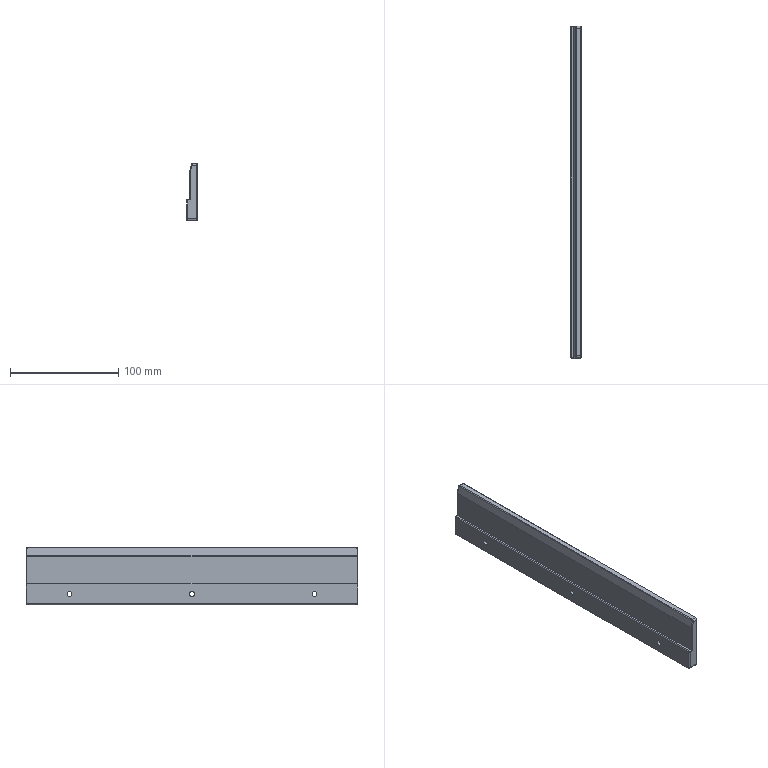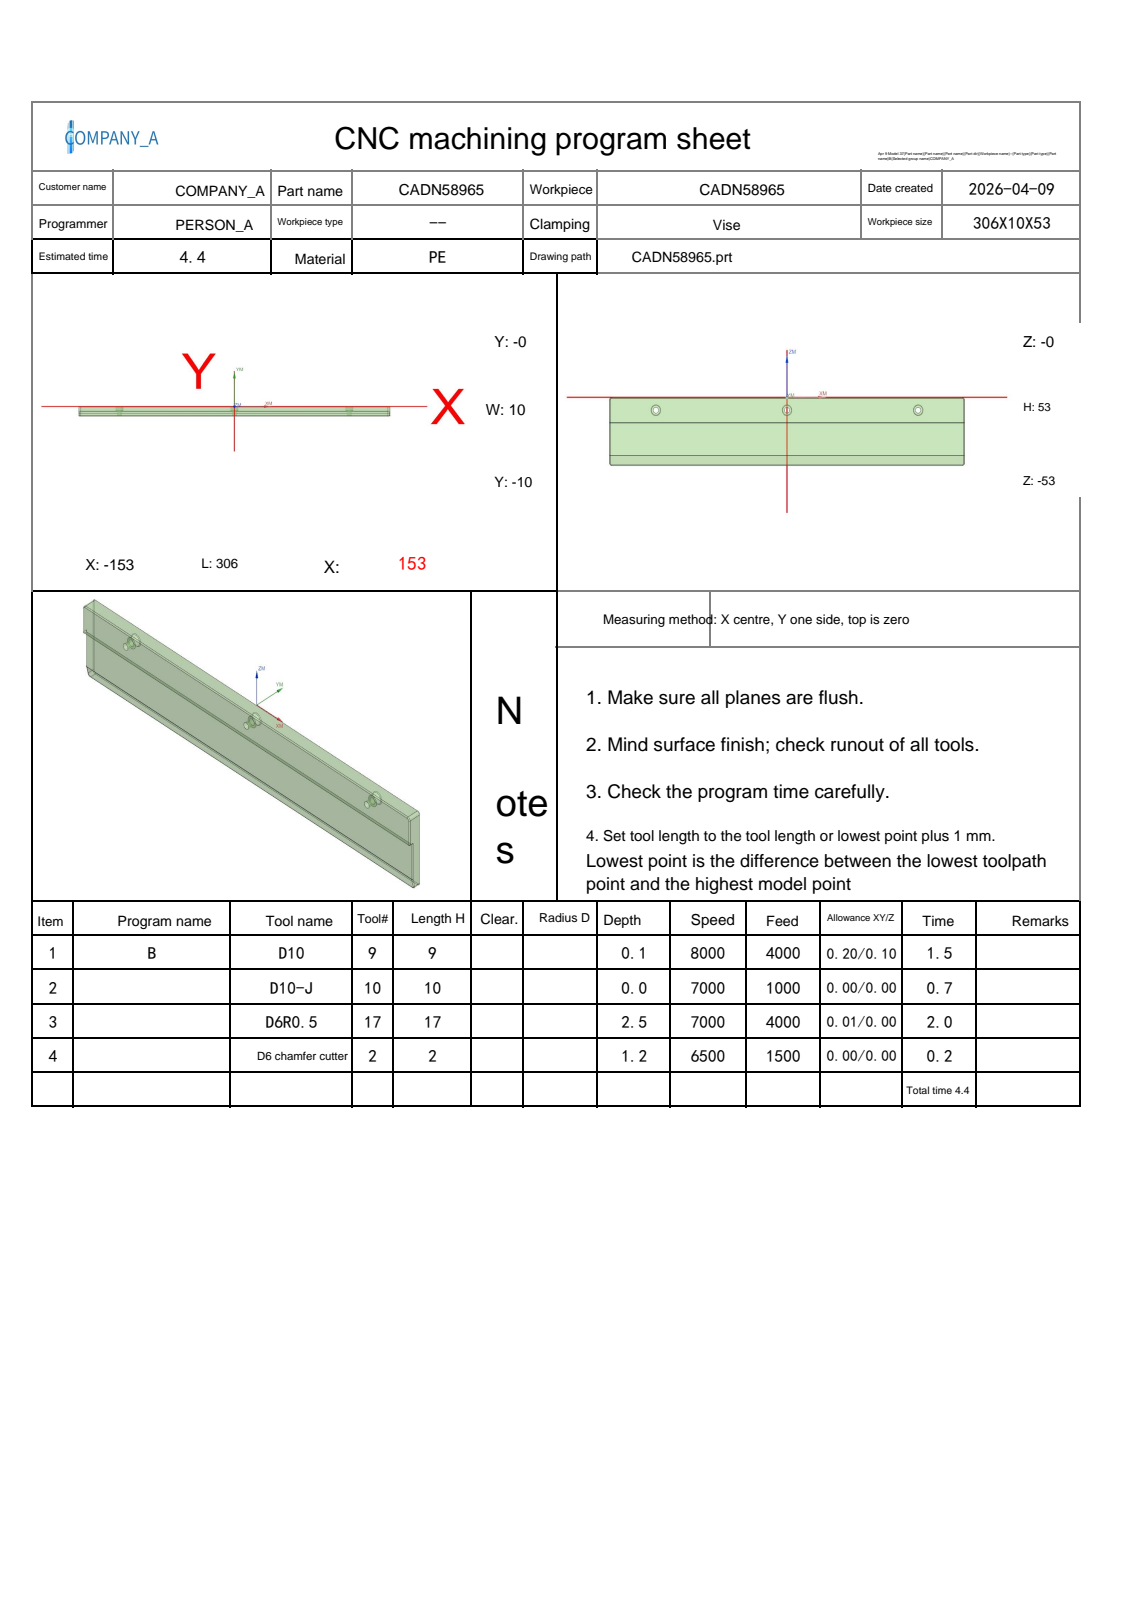NC program | NX | posted by the shop | part box 10 x 306 x 53 mm
Whole program:
%
O0001
(Machine time: 5.28 MIN)
(===Total Tool:4===)
(T9=D10     D=10.  R=0.   D-  H09 Z=0.1   )
(T10=D10-J  D=10.  R=0.   D-  H10 Z=-0.   )
(T17=D6R0.5 D=6.   R=0.5  D-  H17 Z=-2.5  )
(T2=D6 chamfer cutter   D=6.   R=0.   D-  H02 Z=-1.2  )
G80 G90 G17 G49 G40
G91 G28 Z0
M01
N1 T09 M06
(D10  D=10. R=0. H=09 ce=0.20 di=0.10)
G00 G90 G54 X-170. Y-1.667 M03 S8000
G43 H09 Z50.
M08
Z6.011
G01 Z4.011 F4000.
X-158.
X157.001
G02 X158. Y-2.665 I-.001 J-1.
G01 Y-7.433
G02 X157.1 Y-8.333 I-.9 J0.0
G01 X-158.
X-170.
Z6.011
G00 Z7.5
Y-1.667
Z5.522
G01 Z3.522
X-158.
X157.001
G02 X158. Y-2.665 I-.001 J-1.
G01 Y-7.433
G02 X157.1 Y-8.333 I-.9 J0.0
G01 X-158.
X-170.
Z5.522
G00 Z7.011
Y-1.667
Z5.033
G01 Z3.033
X-158.
X157.001
G02 X158. Y-2.665 I-.001 J-1.
G01 Y-7.433
G02 X157.1 Y-8.333 I-.9 J0.0
G01 X-158.
X-170.
Z5.033
G00 Z6.522
Y-1.667
Z4.544
G01 Z2.544
X-158.
X157.001
G02 X158. Y-2.665 I-.001 J-1.
G01 Y-7.433
G02 X157.1 Y-8.333 I-.9 J0.0
G01 X-158.
X-170.
Z4.544
G00 Z6.033
Y-1.667
Z4.056
G01 Z2.056
X-158.
X157.001
G02 X158. Y-2.665 I-.001 J-1.
G01 Y-7.433
G02 X157.1 Y-8.333 I-.9 J0.0
G01 X-158.
X-170.
Z4.056
G00 Z5.544
Y-1.667
Z3.567
G01 Z1.567
X-158.
X157.001
G02 X158. Y-2.665 I-.001 J-1.
G01 Y-7.433
G02 X157.1 Y-8.333 I-.9 J0.0
G01 X-158.
X-170.
Z3.567
G00 Z5.056
Y-1.667
Z3.078
G01 Z1.078
X-158.
X157.001
G02 X158. Y-2.665 I-.001 J-1.
G01 Y-7.433
G02 X157.1 Y-8.333 I-.9 J0.0
G01 X-158.
X-170.
Z3.078
G00 Z4.567
Y-1.667
Z2.589
G01 Z.589
X-158.
X157.001
G02 X158. Y-2.665 I-.001 J-1.
G01 Y-7.433
G02 X157.1 Y-8.333 I-.9 J0.0
G01 X-158.
X-170.
Z2.589
G00 Z4.078
Y-1.667
Z2.1
G01 Z.1
X-158.
X157.001
G02 X158. Y-2.665 I-.001 J-1.
G01 Y-7.433
G02 X157.1 Y-8.333 I-.9 J0.0
G01 X-158.
X-170.
Z2.1
G00 Z50.
G91 G28 Z0.0
M05
M09
G91 G28 Z0.0
M01
N2 T10 M06
(D10-J  D=10. R=0. H=10 ce=0.00 di=0.00)
G00 G90 G54 X-170. Y-1.667 M03 S7000
G43 H10 Z50.
M08
Z2.
G01 Z0.0 F1000.
X-158.
X158.
Y-8.333
X-158.
X-170.
Z2.
G00 Z50.
G91 G28 Z0.0
M05
M09
G91 G28 Z0.0
M01
N3 T17 M06
(D6R0.5  D=6. R=0.5 H=17 ce=0.01 di=0.00)
G00 G90 G54 X146.733 Y5.097 M03 S7000
G43 H17 Z14.5
M08
Z.492
G01 Z-.008 F4000.
X146.742 Y4.929
G03 X149.738 Y2.091 I2.996 J.162
G01 X149.9 Y2.096
G02 X150.286 Y2.106 I.386 J-7.122
X151.984 Y1.901 I0.0 J-7.133
X153.705 Y-.5 I-.992 J-2.528
G01 Y-9.131
G02 X151.026 Y-11.872 I-2.742 J0.0
G01 X149.898 Y-11.898
Y-11.934 Z-.012
Y-11.964 Z-.017
X150.946 Y-11.953
X150.968
G03 X153.8 Y-9.25 I0.0 J2.834
G01 Y-.5
G03 X151.092 Y2.121 I-2.729 J-.111
G01 X149.804 Y2.131
X149.834 Y2.172 Z-.028
G02 X150.411 Y2.191 I.576 J-8.894
X151.504 Y2.123 I0.0 J-8.912
X153.883 Y-.5 I-.333 J-2.692
G01 Y-9.25
G02 X151.052 Y-12.006 I-2.873 J.119
G01 X149.898 Y-12.023
Y-12.078 Z-.041
G03 X150.423 Y-12.099 I.524 J6.576
X151.594 Y-11.994 I0.0 J6.596
X153.962 Y-9.25 I-.512 J2.835
G01 Y-.5
G03 X151.189 Y2.195 I-2.793 J-.1
G01 X149.858 Y2.205
X149.888 Y2.245 Z-.061
X151.292 Y2.232
X151.551 Y2.203
G02 X154.057 Y-.5 I-.324 J-2.813
G01 Y-9.25
G02 X151.566 Y-12.081 I-2.965 J.097
G01 X151.292 Y-12.126
X149.898 Y-12.144
Y-12.181 Z-.073
Y-12.214 Z-.085
G03 X150.386 Y-12.227 I.487 J8.645
X151.527 Y-12.152 I0.0 J8.658
X154.157 Y-9.25 I-.4 J3.005
G01 Y-.5
G03 X151.824 Y2.193 I-2.814 J-.081
X150.477 Y2.309 I-1.347 J-7.773
X149.851 Y2.284 I0.0 J-7.888
G01 X149.881 Y2.322 Z-.114
X151.292 Y2.318
X151.638 Y2.279
G02 X154.256 Y-.5 I-.284 J-2.889
G01 Y-9.25
G02 X151.638 Y-12.208 I-3.105 J.111
X150.43 Y-12.298 I-1.209 J8.067
X149.898 Y-12.281 I0.0 J8.157
G01 Y-12.315 Z-.13
Y-12.346 Z-.146
X151.292 Y-12.322
X151.536 Y-12.295
G03 X154.352 Y-9.25 I-.353 J3.151
G01 Y-.491
G03 X153.21 Y1.704 I-2.681 J0.0
X151.169 Y2.355 I-2.064 J-2.943
G01 X149.879 Y2.363
X149.872 Y2.399 Z-.182
X151.292 Y2.388
X151.638 Y2.35
G02 X153.654 Y1.412 I-.307 J-3.293
X154.447 Y-.484 I-1.87 J-1.895
G01 Y-9.25
G02 X151.821 Y-12.303 I-3.201 J.098
X150.434 Y-12.428 I-1.387 J7.59
X149.898 Y-12.41 I0.0 J7.716
G01 Y-12.471 Z-.222
X149.908 Y-12.467
X150.946
X150.989
G03 X152.676 Y-12.089 I0.0 J3.952
X154.54 Y-9.25 I-1.352 J2.919
G01 Y-.479
G03 X153.649 Y1.515 I-2.678 J0.0
X151.638 Y2.392 I-2.331 J-2.601
G01 X151.292 Y2.428
X149.899 Y2.439
X149.9 Y2.461 Z-.244
Y2.483 Z-.265
X151.292 Y2.471
X151.569 Y2.444
G02 X153.368 Y1.821 I-.398 J-4.06
X154.631 Y-.5 I-1.565 J-2.355
G01 Y-9.25
G02 X153.73 Y-11.418 I-3.06 J0.0
X151.138 Y-12.512 I-2.648 J2.66
G01 X149.898 Y-12.53
Y-12.559 Z-.289
Y-12.587 Z-.312
X151.097 Y-12.571
G03 X152.95 Y-12.103 I-.055 J4.119
X154.72 Y-9.25 I-1.528 J2.924
G01 Y-.5
G03 X153.318 Y1.923 I-2.794 J0.0
X151.118 Y2.519 I-2.237 J-3.895
G01 X149.903 Y2.53
X149.906 Y2.555 Z-.338
X149.908 Y2.58 Z-.363
X151.292 Y2.568
G02 X153.368 Y1.956 I-.316 J-4.895
X154.807 Y-.5 I-1.439 J-2.493
G01 Y-9.25
G02 X153.009 Y-12.151 I-3.352 J.069
X151.111 Y-12.628 I-1.942 J3.713
G01 X149.898 Y-12.641
Y-12.667 Z-.39
Y-12.692 Z-.417
G03 X150.415 Y-12.703 I.517 J12.433
X151.472 Y-12.658 I0.0 J12.443
X153.368 Y-12.007 I-.35 J4.108
X154.892 Y-9.25 I-1.825 J2.808
G01 Y-.5
G03 X153.368 Y2.011 I-2.871 J-.025
X151.292 Y2.622 I-2.436 J-4.444
G01 X149.908 Y2.634
Y2.663 Z-.445
Y2.691 Z-.474
X151.292 Y2.678
G02 X153.714 Y1.857 I-.382 J-5.109
X154.975 Y-.5 I-1.614 J-2.379
G01 Y-9.25
G02 X153.714 Y-11.833 I-3.359 J.041
X151.638 Y-12.689 I-2.484 J3.078
X150.405 Y-12.75 I-1.233 J12.337
X149.898 Y-12.74 I0.0 J12.398
G01 Y-12.763 Z-.504
Y-12.785 Z-.535
G03 X150.442 Y-12.797 I.544 J12.121
X151.638 Y-12.738 I0.0 J12.133
X153.46 Y-12.096 I-.459 J4.205
X155.055 Y-9.25 I-1.831 J2.896
G01 Y-.5
G03 X153.714 Y1.926 I-2.921 J-.03
X151.638 Y2.704 I-2.97 J-4.773
X150.446 Y2.764 I-1.193 J-11.794
X149.908 Y2.752 I0.0 J-11.854
G01 X149.913 Y2.784 Z-.566
X149.917 Y2.815 Z-.598
G02 X150.445 Y2.827 I.527 J-11.795
X151.638 Y2.767 I0.0 J-11.806
X153.901 Y1.852 I-.903 J-5.488
X155.133 Y-.499 I-1.627 J-2.351
G01 Y-9.25
G02 X153.377 Y-12.219 I-3.478 J.053
X151.165 Y-12.815 I-2.253 J3.953
G01 X149.898 Y-12.827
Y-12.846 Z-.631
Y-12.865 Z-.665
G03 X150.361 Y-12.871 I.463 J17.439
X151.638 Y-12.824 I0.0 J17.445
X153.672 Y-12.096 I-.373 J4.245
X155.208 Y-9.25 I-1.952 J2.891
G01 Y-.5
G03 X154.06 Y1.797 I-2.906 J-.017
G01 X153.714 Y2.029
G03 X151.638 Y2.831 I-2.982 J-4.63
X150.368 Y2.889 I-1.27 J-13.825
X149.923 Y2.882 I0.0 J-13.884
G01 X149.925 Y2.917 Z-.7
X149.926 Y2.952 Z-.734
G02 X150.359 Y2.959 I.432 J-13.383
X151.638 Y2.897 I0.0 J-13.39
X153.714 Y2.084 I-.885 J-5.312
X155.28 Y-.5 I-1.417 J-2.625
G01 Y-9.25
G02 X154.06 Y-11.869 I-3.504 J.038
X152.676 Y-12.644 I-2.556 J2.941
X151.292 Y-12.89 I-1.645 J5.257
X150.42 Y-12.904 I-.872 J26.727
X149.898 Y-12.899 I0.0 J26.742
G01 Y-12.914 Z-.77
Y-12.928 Z-.805
G03 X150.335 Y-12.931 I.437 J33.827
X151.292 Y-12.917 I0.0 J33.83
X153.368 Y-12.404 I-.121 J4.941
X155.348 Y-9.25 I-1.618 J3.213
G01 Y-.5
G03 X153.778 Y2.098 I-3.007 J-.044
X151.638 Y2.965 I-3.031 J-4.408
X150.35 Y3.029 I-1.289 J-12.859
X149.93 Y3.022 I0.0 J-12.923
G01 X149.931 Y3.058 Z-.84
X149.933 Y3.093 Z-.876
G02 X150.331 Y3.099 I.398 J-12.767
X151.638 Y3.032 I0.0 J-12.774
X153.864 Y2.098 I-.94 J-5.359
X154.681 Y1.419 I-1.849 J-3.054
X155.41 Y-.498 I-2.152 J-1.916
G01 Y-9.25
G02 X153.387 Y-12.442 I-3.616 J.055
X151.638 Y-12.92 I-2.076 J4.154
X150.426 Y-12.96 I-1.213 J18.383
X149.898 Y-12.953 I0.0 J18.423
G01 Y-12.963 Z-.911
Y-12.973 Z-.946
G03 X150.42 Y-12.979 I.522 J20.386
X151.638 Y-12.943 I0.0 J20.392
X153.472 Y-12.442 I-.274 J4.611
X155.469 Y-9.25 I-1.628 J3.239
G01 Y-.5
G03 X154.411 Y1.752 I-2.982 J-.026
X153.022 Y2.646 I-5.027 J-6.285
X150.946 Y3.158 I-2.116 J-4.119
G01 X149.936 Y3.164
X149.938 Y3.199 Z-.982
X149.939 Y3.234 Z-1.017
X150.946 Y3.228
G02 X153.022 Y2.707 I-.068 J-4.665
X154.406 Y1.8 I-3.808 J-7.318
X155.523 Y-.5 I-1.845 J-2.317
G01 Y-9.25
G02 X154.099 Y-12.096 I-3.655 J.05
X152.33 Y-12.872 I-2.554 J3.415
X151.108 Y-12.985 I-1.222 J6.53
G01 X149.908
X149.898 Y-12.988
Y-12.999 Z-1.088
X149.908 Y-12.993
X151.292 Y-12.99
X151.294
G03 X152.538 Y-12.853 I0.0 J5.701
X154.062 Y-12.172 I-.915 J4.094
X155.573 Y-9.25 I-2.174 J2.976
G01 Y-.499
G03 X154.545 Y1.728 I-2.926 J0.0
X153.022 Y2.768 I-5.624 J-6.598
X150.946 Y3.299 I-2.156 J-4.104
G01 X149.942 Y3.305
X149.944 Y3.341 Z-1.123
X149.946 Y3.376 Z-1.159
X150.946 Y3.37
G02 X153.085 Y2.791 I-.077 J-4.52
X154.406 Y1.887 I-4.192 J-7.55
G01 X154.576 Y1.752
G02 X155.62 Y-.5 I-1.965 J-2.279
G01 Y-9.25
G02 X153.699 Y-12.442 I-3.679 J.04
X151.638 Y-12.988 I-2.176 J4.051
X150.446 Y-13.005 I-1.192 J41.959
X149.908 Y-13.001 I0.0 J41.976
G01 X149.898 Y-13.007
Y-13.01 Z-1.229
X151.292 Y-13.005
X151.638 Y-12.994
X151.984 Y-12.977
G03 X153.719 Y-12.466 I-.38 J4.491
X155.663 Y-9.25 I-1.763 J3.262
G01 Y-.5
G03 X155.098 Y1.236 I-3.045 J-.031
X154.191 Y2.098 I-3.384 J-2.649
X152.676 Y3.053 I-4.536 J-5.518
X150.946 Y3.441 I-1.784 J-3.908
G01 X149.949 Y3.446
X150.063 Y3.515 Z-1.3
X150.946 Y3.512
G02 X153.022 Y2.941 I-.077 J-4.344
X154.406 Y1.966 I-4.582 J-7.972
G01 X154.646 Y1.764
G02 X155.444 Y.709 I-1.935 J-2.293
X155.703 Y-.5 I-2.919 J-1.258
G01 Y-9.25
G02 X155.619 Y-10.019 I-5.658 J.232
X153.368 Y-12.659 I-3.658 J.839
X151.984 Y-12.987 I-1.709 J4.125
X150.598 Y-13.018 I-1.387 J31.571
X149.903 Y-13.01 I0.0 J31.601
G01 Z-1.371
X151.638 Y-13.007
X151.878 Y-12.999
G03 X153.733 Y-12.514 I-.135 J4.307
X155.654 Y-10.019 I-1.728 J3.317
X155.74 Y-9.25 I-4.53 J.897
G01 Y-.5
G03 X154.752 Y1.709 I-3.03 J-.03
X153.213 Y2.886 I-8.157 J-9.068
X151.243 Y3.563 I-2.352 J-3.641
X150.623 Y3.59 I-.62 J-7.028
X150.352 Y3.585 I0.0 J-7.055
G01 X150.506 Y3.604 Z-1.388
X150.66 Y3.621 Z-1.406
X150.814 Y3.638 Z-1.424
X150.968 Y3.654 Z-1.442
G02 X153.022 Y3.056 I-.097 J-4.16
X154.343 Y2.098 I-5.431 J-8.877
G01 X154.406 Y2.038
X154.752 Y1.744
G02 X155.775 Y-.5 I-1.99 J-2.262
G01 Y-9.25
G02 X153.751 Y-12.533 I-3.732 J.036
X151.984 Y-12.999 I-1.956 J3.833
G01 X151.638 Y-13.01
X149.903
Z-1.514
X151.638
X151.984 Y-13.002
G03 X153.836 Y-12.51 I-.112 J4.15
X155.808 Y-9.25 I-1.76 J3.291
G01 Y-.5
G03 X154.778 Y1.752 I-3.012 J-.015
G01 X154.752 Y1.773
G03 X153.368 Y2.891 I-9.232 J-10.011
X151.984 Y3.574 I-2.735 J-3.796
G01 X152.12 Y3.553 Z-1.534
X152.255 Y3.525 Z-1.553
X152.387 Y3.49 Z-1.572
X152.514 Y3.448 Z-1.592
G02 X153.439 Y2.894 I-2.385 J-5.026
X154.752 Y1.802 I-8.968 J-12.119
G01 X154.814 Y1.752
G02 X155.839 Y-.5 I-1.994 J-2.267
G01 Y-9.25
G02 X153.714 Y-12.595 I-3.742 J.03
X151.984 Y-13.005 I-1.782 J3.664
G01 X151.638 Y-13.01
X149.903
Z-1.674
X151.638
X151.984 Y-13.009
X151.986
G03 X154.752 Y-11.899 I0.0 J4.001
X155.87 Y-9.25 I-2.681 J2.691
G01 Y-.5
G03 X154.842 Y1.752 I-3.003 J-.01
G01 X154.752 Y1.832
G03 X153.368 Y3.004 I-11.822 J-12.558
X152.854 Y3.336 I-2.326 J-3.042
G01 X152.984 Y3.298 Z-1.717
X153.106 Y3.247 Z-1.76
G02 X153.811 Y2.704 I-4.233 J-6.228
G01 X154.06 Y2.488
G02 X154.988 Y1.642 I-15.354 J-17.779
X155.898 Y-.495 I-2.055 J-2.137
G01 Y-9.25
G02 X154.17 Y-12.391 I-3.772 J.03
X152.015 Y-13.01 I-2.155 J3.44
G01 X151.984
X149.903
Z-1.849
X151.984
X152.046
G03 X153.294 Y-12.817 I0.0 J4.126
X155.924 Y-9.25 I-1.139 J3.592
G01 Y-.493
G03 X155.004 Y1.653 I-2.962 J0.0
G01 X154.899 Y1.752
G03 X153.3 Y3.166 I-13.874 J-14.074
G01 X153.442 Y3.114 Z-1.942
G02 X154.927 Y1.752 I-20.346 J-23.681
G01 X155.013 Y1.671
G02 X155.947 Y-.497 I-2.049 J-2.168
G01 Y-9.25
G02 X152.33 Y-13. I-3.778 J.025
G01 X151.984 Y-13.01
X149.903
Z-2.037
X151.984
X152.043
G03 X152.724 Y-12.964 I0.0 J4.977
X155.967 Y-9.25 I-.52 J3.727
G01 Y-.5
G03 X155.098 Y1.611 I-3.006 J-.003
X153.547 Y3.069 I-37.068 J-37.895
G01 X153.647 Y3.017 Z-2.134
G02 X155.098 Y1.629 I-51.25 J-55.077
X155.983 Y-.5 I-2.134 J-2.135
G01 Y-9.25
G02 X153.478 Y-12.788 I-3.775 J.017
X152.33 Y-13.004 I-1.381 J4.177
G01 X151.984 Y-13.01
X149.903
Z-2.225
X152.14
G03 X152.724 Y-12.971 I0.0 J4.416
X155.995 Y-9.25 I-.499 J3.736
G01 Y-.5
G03 X155.098 Y1.642 I-3.036 J-.012
G01 X153.848 Y2.857
X153.725 Y2.976
X153.763 Y2.961 Z-2.317
G03 X155.098 Y1.647 I121.481 J122.038
G02 X156.003 Y-.5 I-2.09 J-2.146
G01 Y-9.25
G02 X155.968 Y-9.704 I-5.192 J.178
X152.252 Y-13.009 I-3.735 J.458
G01 X151.984 Y-13.01
X149.903
Z-2.408
X151.984
X152.33 Y-13.009
G03 X156.008 Y-9.25 I-.093 J3.77
G01 Y-.497
G03 X155.12 Y1.632 I-2.992 J0.0
G01 X153.796 Y2.94
X153.83 Y2.92 Z-2.5
X155.141 Y1.615
G02 X156.01 Y-.49 I-2.137 J-2.113
G01 X156.009 Y-9.326
G02 X152.33 Y-13.009 I-3.759 J.076
G01 X151.984 Y-13.01
X149.903
G00 Z14.5
X-146.998 Y-14.898
Z.492
G01 Z-.008
Y-14.896
G03 X-149.898 Y-11.898 I-3. J0.0
G01 X-151.112 Y-11.858
G02 X-153.705 Y-9.25 I.089 J2.681
G01 Y-.5
G02 X-151.645 Y1.988 I2.632 J-.083
X-150.432 Y2.121 I1.213 J-5.45
X-149.9 Y2.096 I0.0 J-5.583
G01 X-149.804 Y2.131 Z-.017
X-151.092 Y2.121
G03 X-153.8 Y-.5 I.022 J-2.732
G01 Y-9.25
G03 X-150.981 Y-11.953 I2.819 J.118
G01 X-150.946
X-149.898 Y-11.964
Y-12.023 Z-.028
X-151.108 Y-11.996
G02 X-153.883 Y-9.25 I.063 J2.839
G01 Y-.5
G02 X-151.504 Y2.123 I2.711 J-.068
X-150.411 Y2.191 I1.093 J-8.845
X-149.834 Y2.172 I0.0 J-8.912
G01 X-149.858 Y2.205 Z-.041
X-151.292 Y2.194
X-151.638 Y2.146
G03 X-153.962 Y-.5 I.448 J-2.737
G01 Y-9.25
G03 X-151.603 Y-11.993 I2.873 J.085
X-150.423 Y-12.099 I1.181 J6.49
X-149.898 Y-12.078 I0.0 J6.596
G01 Y-12.113 Z-.051
Y-12.144 Z-.061
X-151.292 Y-12.126
X-151.57 Y-12.081
G02 X-154.057 Y-9.25 I.473 J2.923
G01 Y-.5
G02 X-151.551 Y2.203 I2.829 J-.11
G01 X-151.292 Y2.232
X-149.888 Y2.245
X-149.851 Y2.284 Z-.085
G03 X-150.477 Y2.309 I-.626 J-7.864
X-151.824 Y2.193 I0.0 J-7.888
X-154.157 Y-.5 I.481 J-2.774
G01 Y-9.25
G03 X-151.528 Y-12.152 I3.029 J.102
X-150.386 Y-12.227 I1.143 J8.583
X-149.898 Y-12.214 I0.0 J8.658
G01 Y-12.249 Z-.099
Y-12.281 Z-.114
G02 X-150.43 Y-12.298 I-.531 J8.139
X-151.638 Y-12.208 I0.0 J8.157
X-154.256 Y-9.25 I.487 J3.067
G01 Y-.5
G02 X-151.638 Y2.279 I2.901 J-.111
G01 X-151.292 Y2.318
X-149.881 Y2.322
X-149.88 Y2.346 Z-.13
X-149.879 Y2.363 Z-.146
X-151.177 Y2.355
G03 X-152.813 Y1.941 I.022 J-3.527
G01 X-153.022 Y1.83
G03 X-154.352 Y-.5 I1.471 J-2.384
G01 Y-9.25
G03 X-151.536 Y-12.295 I3.169 J.107
G01 X-151.292 Y-12.322
X-149.898 Y-12.346
Y-12.379 Z-.164
Y-12.41 Z-.182
G02 X-150.434 Y-12.428 I-.536 J7.697
X-151.821 Y-12.303 I0.0 J7.716
X-154.447 Y-9.25 I.576 J3.151
G01 Y-.5
G02 X-151.984 Y2.296 I2.947 J-.113
X-150.454 Y2.417 I1.531 J-9.63
X-149.872 Y2.399 I0.0 J-9.751
G01 X-149.899 Y2.439 Z-.222
X-151.292 Y2.428
X-151.638 Y2.392
G03 X-153.022 Y1.965 I.419 J-3.818
X-154.54 Y-.5 I1.31 J-2.506
G01 Y-9.25
G03 X-154.147 Y-10.711 I3.201 J.077
X-151.55 Y-12.426 I2.984 J1.696
G01 X-151.292 Y-12.455
X-149.898 Y-12.471
Y-12.502 Z-.244
Y-12.53 Z-.265
X-151.292 Y-12.509
X-151.638 Y-12.475
G02 X-154.051 Y-11.033 I.486 J3.551
X-154.631 Y-9.251 I2.45 J1.782
G01 Y-.5
G02 X-153.023 Y2.023 I2.85 J-.043
X-151.097 Y2.473 I1.962 J-4.053
G01 X-149.9 Y2.483
X-149.901 Y2.506 Z-.289
X-149.903 Y2.53 Z-.312
X-151.292 Y2.518
G03 X-153.293 Y1.937 I.252 J-4.599
X-154.72 Y-.5 I1.366 J-2.436
G01 Y-9.26
G03 X-154.343 Y-10.714 I2.996 J0.0
X-151.638 Y-12.531 I3.13 J1.738
G01 X-151.292 Y-12.568
X-149.898 Y-12.587
Y-12.614 Z-.338
Y-12.641 Z-.363
X-151.292 Y-12.626
X-151.638 Y-12.591
G02 X-154.039 Y-11.315 I.466 J3.773
X-154.807 Y-9.263 I2.356 J2.052
G01 Y-.5
G02 X-153.368 Y1.956 I2.878 J-.037
X-150.964 Y2.58 I2.404 J-4.316
G01 X-150.946
X-149.908
Y2.607 Z-.39
Y2.634 Z-.417
X-150.946
G03 X-153.368 Y2.011 I.009 J-5.051
X-154.892 Y-.5 I1.347 J-2.535
G01 Y-9.25
G03 X-154.068 Y-11.403 I3.377 J.059
X-151.638 Y-12.642 I2.875 J2.635
X-150.415 Y-12.703 I1.223 J12.383
X-149.898 Y-12.692 I0.0 J12.443
G01 Y-12.717 Z-.445
Y-12.74 Z-.474
G02 X-150.433 Y-12.754 I-.535 J10.139
X-151.84 Y-12.656 I0.0 J10.153
X-154.419 Y-11.062 I.522 J3.728
X-154.975 Y-9.275 I2.597 J1.787
G01 Y-.5
G02 X-153.864 Y1.752 I2.895 J-.028
X-150.946 Y2.691 I2.938 J-4.126
G01 X-149.908
Y2.721 Z-.504
Y2.752 Z-.535
X-150.946
G03 X-153.837 Y1.834 I.044 J-5.15
X-155.055 Y-.492 I1.613 J-2.327
G01 Y-9.25
G03 X-153.46 Y-12.096 I3.426 J.05
X-151.638 Y-12.738 I2.28 J3.563
X-150.442 Y-12.797 I1.196 J12.074
X-149.898 Y-12.785 I0.0 J12.133
G01 Y-12.806 Z-.566
Y-12.827 Z-.598
X-151.165 Y-12.815
G02 X-153.377 Y-12.219 I.041 J4.549
X-155.133 Y-9.25 I1.722 J3.022
G01 Y-.499
G02 X-153.901 Y1.852 I2.859 J0.0
X-151.638 Y2.767 I3.165 J-4.574
X-150.4 Y2.824 I1.238 J-13.324
X-149.917 Y2.815 I0.0 J-13.381
G01 X-149.92 Y2.849 Z-.631
X-149.923 Y2.882 Z-.665
G03 X-150.36 Y2.889 I-.436 J-14.162
X-151.638 Y2.831 I0.0 J-14.169
X-153.714 Y2.029 I.906 J-5.431
G01 X-154.06 Y1.797
G03 X-155.208 Y-.5 I1.759 J-2.314
G01 Y-9.25
G03 X-154.107 Y-11.75 I3.496 J.047
X-151.638 Y-12.824 I2.824 J3.117
G01 X-151.292 Y-12.851
X-149.898 Y-12.865
Y-12.882 Z-.7
Y-12.899 Z-.734
G02 X-150.42 Y-12.904 I-.522 J26.736
X-151.292 Y-12.89 I0.0 J26.742
X-153.191 Y-12.442 I.207 J5.129
X-155.09 Y-10.365 I1.569 J3.34
X-155.28 Y-9.25 I3.839 J1.228
G01 Y-.5
G02 X-153.714 Y2.084 I2.982 J-.041
X-151.292 Y2.933 I2.871 J-4.309
G01 X-150.946 Y2.949
X-150.6 Y2.951
X-149.926 Y2.952
X-149.928 Y2.987 Z-.77
X-149.93 Y3.022 Z-.805
G03 X-150.342 Y3.029 I-.412 J-13.099
X-151.638 Y2.964 I0.0 J-13.105
X-153.778 Y2.098 I.889 J-5.271
X-155.348 Y-.5 I1.437 J-2.642
G01 Y-9.25
G03 X-153.368 Y-12.404 I3.597 J.06
X-151.292 Y-12.917 I2.197 J4.427
X-150.335 Y-12.931 I.958 J33.816
X-149.898 Y-12.928 I0.0 J33.83
G01 Y-12.941 Z-.84
Y-12.953 Z-.876
G02 X-150.426 Y-12.96 I-.528 J18.415
X-151.638 Y-12.92 I0.0 J18.423
X-153.387 Y-12.442 I.328 J4.632
X-155.41 Y-9.25 I1.593 J3.247
G01 Y-.497
G02 X-154.337 Y1.753 I2.892 J0.0
X-152.678 Y2.743 I4.303 J-5.323
X-150.986 Y3.088 I1.715 J-4.093
G01 X-149.933 Y3.093
X-149.934 Y3.128 Z-.911
X-149.936 Y3.164 Z-.946
X-150.946 Y3.158
G03 X-153.022 Y2.646 I.042 J-4.639
X-154.411 Y1.752 I3.637 J-7.177
X-155.469 Y-.5 I1.924 J-2.278
G01 Y-9.25
G03 X-153.472 Y-12.442 I3.625 J.047
X-151.638 Y-12.943 I2.108 J4.11
X-150.42 Y-12.979 I1.218 J20.356
X-149.898 Y-12.973 I0.0 J20.392
G01 Y-12.981 Z-.982
Y-12.988 Z-1.017
X-151.292 Y-12.983
X-151.638 Y-12.963
G02 X-153.555 Y-12.442 I.245 J4.686
X-155.434 Y-10.019 I1.706 J3.262
X-155.523 Y-9.25 I5.89 J1.073
G01 Y-.5
G02 X-154.406 Y1.8 I2.961 J-.017
X-153.022 Y2.707 I5.198 J-6.421
X-150.946 Y3.228 I2.147 J-4.154
G01 X-149.939 Y3.234
X-149.941 Y3.27 Z-1.053
X-149.943 Y3.305 Z-1.088
X-150.946 Y3.299
G03 X-153.022 Y2.768 I.083 J-4.646
X-154.546 Y1.727 I4.099 J-7.635
X-155.573 Y-.498 I1.897 J-2.225
G01 Y-9.25
G03 X-155.444 Y-10.19 I5.382 J.259
X-153.627 Y-12.442 I3.564 J1.016
X-151.638 Y-12.981 I2.207 J4.207
X-150.45 Y-12.997 I1.189 J44.173
X-149.908 Y-12.993 I0.0 J44.189
G01 X-149.898 Y-12.999
Y-13.007 Z-1.159
X-149.908 Y-13.001
X-150.946
X-151.048 Y-13.002
G02 X-151.984 Y-12.963 I0.0 J11.299
X-154.106 Y-12.184 I.382 J4.32
X-155.62 Y-9.25 I2.162 J2.973
G01 Y-.5
G02 X-154.576 Y1.752 I3.005 J-.025
G01 X-154.279 Y1.988
G02 X-153.064 Y2.802 I5.454 J-6.832
X-150.946 Y3.37 I2.197 J-3.962
G01 X-149.946 Y3.376
X-149.947 Y3.411 Z-1.194
X-149.949 Y3.446 Z-1.229
X-150.908 Y3.44
G03 X-153.164 Y2.797 I.027 J-4.369
G01 X-153.714 Y2.46
G03 X-154.618 Y1.752 I9.575 J-13.152
X-155.663 Y-.5 I1.949 J-2.273
G01 Y-9.25
G03 X-153.719 Y-12.466 I3.707 J.046
X-151.984 Y-12.977 I2.114 J3.981
G01 X-151.638 Y-12.994
X-151.292 Y-13.005
X-149.898 Y-13.01
X-149.903 Z-1.3
G02 X-150.598 Y-13.018 I-.695 J31.58
X-151.844 Y-12.993 I0.0 J31.587
X-153.718 Y-12.498 I.176 J4.46
X-154.984 Y-11.403 I1.805 J3.369
X-155.619 Y-10.019 I3.005 J2.214
X-155.703 Y-9.25 I5.574 J1.
G01 Y-.5
G02 X-155.442 Y.713 I3.176 J-.049
X-154.636 Y1.772 I2.779 J-1.28
G01 X-154.406 Y1.966
G02 X-153.022 Y2.941 I5.96 J-6.989
X-150.946 Y3.511 I2.152 J-3.776
G01 X-150.062 Y3.515
X-150.204 Y3.551 Z-1.335
X-150.346 Y3.584 Z-1.371
G03 X-150.609 Y3.588 I-.263 J-7.343
X-151.241 Y3.561 I0.0 J-7.348
X-153.214 Y2.886 I.371 J-4.306
X-154.752 Y1.709 I6.619 J-10.244
X-155.74 Y-.5 I2.041 J-2.239
G01 Y-9.25
G03 X-155.654 Y-10.019 I4.616 J.129
X-154.406 Y-12.067 I3.667 J.829
X-153.742 Y-12.514 I2.868 J3.548
X-151.686 Y-13.007 I2.056 J4.042
G01 X-151.638
X-151.292 Y-13.01
X-149.903
Z-1.442
X-151.638
X-151.984 Y-12.999
G02 X-154.143 Y-12.296 I.158 J4.151
X-155.775 Y-9.25 I2.083 J3.076
G01 Y-.5
G02 X-154.752 Y1.744 I3.015 J-.019
G01 X-154.406 Y2.038
X-154.343 Y2.098
G02 X-153.022 Y3.056 I6.738 J-7.901
X-150.943 Y3.652 I2.142 J-3.546
G01 X-151.093 Y3.657 Z-1.452
X-151.243 Y3.655 Z-1.462
X-151.394 Y3.65 Z-1.473
X-151.544 Y3.643 Z-1.483
X-151.694 Y3.627 Z-1.494
X-151.84 Y3.604 Z-1.504
X-151.984 Y3.574 Z-1.514
G03 X-153.368 Y2.891 I1.355 J-4.488
X-154.752 Y1.773 I7.846 J-11.126
G01 X-154.778 Y1.752
G03 X-155.808 Y-.5 I1.984 J-2.268
G01 Y-9.25
G03 X-155.501 Y-10.711 I3.908 J.056
X-154.133 Y-12.334 I3.501 J1.563
X-151.984 Y-13.002 I2.257 J3.471
G01 X-151.638 Y-13.01
X-149.903
Z-1.592
X-151.638
X-151.984 Y-13.005
G02 X-154.495 Y-12.096 I.044 J4.041
X-155.444 Y-10.902 I2.51 J2.969
X-155.839 Y-9.25 I3.484 J1.706
G01 Y-.5
G02 X-154.814 Y1.752 I3.02 J-.015
G01 X-154.752 Y1.802
G02 X-153.439 Y2.894 I10.275 J-11.019
X-152.514 Y3.448 I3.308 J-4.47
G01 X-152.631 Y3.419 Z-1.619
X-152.746 Y3.384 Z-1.647
X-152.854 Y3.336 Z-1.674
G03 X-153.368 Y3.004 I1.812 J-3.376
X-154.461 Y2.098 I9.259 J-12.272
G01 X-154.752 Y1.832
X-154.842 Y1.752
G03 X-155.87 Y-.5 I1.978 J-2.263
G01 Y-9.25
G03 X-155.098 Y-11.506 I3.81 J.044
X-152.217 Y-12.998 I3.066 J2.393
G01 X-151.984 Y-13.009
X-149.903 Y-13.01
Z-1.76
X-151.984
X-152.234 Y-13.
G02 X-155.535 Y-10.844 I.155 J3.842
X-155.898 Y-9.25 I3.603 J1.658
G01 Y-.5
G02 X-155.146 Y1.483 I3.036 J-.017
X-154.06 Y2.488 I13.697 J-13.707
G01 X-153.811 Y2.704
G02 X-153.106 Y3.247 I4.929 J-5.676
G01 X-153.208 Y3.213 Z-1.805
X-153.3 Y3.166 Z-1.849
G03 X-154.42 Y2.204 I9.652 J-12.368
G01 X-154.991 Y1.665
G03 X-155.924 Y-.498 I2.043 J-2.163
G01 Y-9.25
G03 X-155.623 Y-10.711 I4.024 J.066
X-152.33 Y-12.998 I3.5 J1.525
G01 X-151.984 Y-13.01
X-149.903
Z-1.942
X-151.984
X-152.33 Y-13.
G02 X-155.947 Y-9.25 I.161 J3.775
G01 Y-.494
G02 X-155.069 Y1.613 I2.967 J0.0
X-153.442 Y3.114 I21.884 J-22.08
G01 X-153.547 Y3.069 Z-2.037
G03 X-155.098 Y1.612 I36.472 J-40.382
X-155.967 Y-.5 I2.145 J-2.117
G01 Y-9.25
G03 X-155.669 Y-10.711 I3.92 J.039
X-152.33 Y-13.002 I3.487 J1.503
G01 X-151.984 Y-13.01
X-149.903
Z-2.134
X-151.984
X-152.33 Y-13.004
G02 X-154.752 Y-12.023 I.137 J3.817
X-155.983 Y-9.25 I2.548 J2.791
G01 Y-.5
G02 X-155.098 Y1.63 I3.022 J-.007
X-153.647 Y3.017 I56.991 J-58.182
G01 X-153.725 Y2.976 Z-2.225
G03 X-155.098 Y1.638 I172.382 J-178.295
X-155.995 Y-.5 I2.124 J-2.148
G01 Y-9.25
G03 X-155.79 Y-10.462 I4.023 J.056
X-152.33 Y-13.006 I3.576 J1.239
G01 X-151.984 Y-13.01
X-149.903
Z-2.317
X-151.984
X-152.33 Y-13.008
G02 X-155.999 Y-9.26 I.101 J3.768
G01 X-156.003 Y-9.25
Y-.5
G02 X-155.1 Y1.644 I2.995 J0.0
G03 X-153.764 Y2.96 I-142.973 J146.467
G01 X-153.797 Y2.94 Z-2.408
X-155.121 Y1.629
G03 X-156.008 Y-.498 I2.106 J-2.127
G01 Y-9.25
G03 X-152.33 Y-13.009 I3.771 J.011
G01 X-151.984 Y-13.01
X-149.903
Z-2.5
X-151.984
X-152.33 Y-13.009
G02 X-156.01 Y-9.25 I.08 J3.758
G01 Y-.49
G02 X-155.098 Y1.659 I3.013 J-.01
G01 X-153.961 Y2.791
X-153.831 Y2.919
G00 Z14.5
G00 G90 X155.037 Y-14.103 M03 S7000
Z14.5
Z.486
G01 Z-.014 F4000.
G03 X152.152 Y-11.925 I-2.885 J-.821
G01 X152.1
X151. Y-11.944
X-151.
X-152.101 Y-11.914
Y-11.983 Z-.024
Y-12.033 Z-.034
X-151. Y-12.051
X151.
X152.101 Y-12.04
X152.1 Y-12.099 Z-.049
Y-12.145 Z-.063
X151. Y-12.151
X-151.
X-152.1 Y-12.145
Y-12.198 Z-.081
Y-12.229 Z-.099
X-151. Y-12.247
X151.
X152.1 Y-12.229
Y-12.288 Z-.12
Y-12.328 Z-.142
X151. Y-12.338
X-151.
X-152.101 Y-12.328
Y-12.375 Z-.167
X-152.1 Y-12.415 Z-.192
X-151. Y-12.425
X151.
X152.1 Y-12.413
Y-12.467 Z-.22
Y-12.506 Z-.249
X151. Y-12.508
X-151.
X-152.1 Y-12.506
Y-12.545 Z-.28
X-152.101 Y-12.581 Z-.312
X-151. Y-12.586
X151.
X152.101 Y-12.581
Y-12.618 Z-.347
Y-12.65 Z-.382
X151. Y-12.659
X-151.
X-151.972 Y-12.651
X-152.101 Y-12.65
Y-12.688 Z-.419
Y-12.721 Z-.456
X-151.972
X-151. Y-12.726
X151.
X151.972 Y-12.721
X152.1 Y-12.722
Y-12.756 Z-.496
Y-12.781 Z-.536
X152.059 Y-12.778
X151. Y-12.786
X-151.
X-152.1 Y-12.778
X-152.098 Y-12.812 Z-.579
X-152.096 Y-12.836 Z-.621
X-151. Y-12.84
X151.
X152.096 Y-12.836
Y-12.86 Z-.665
Y-12.88 Z-.709
X151. Y-12.887
X-151.
X-152.096 Y-12.881
X-152.097 Y-12.901 Z-.755
Y-12.925 Z-.801
X-151. Y-12.927
X151.
X152.097 Y-12.924
Y-12.937 Z-.849
Y-12.955 Z-.896
X151. Y-12.959
X-151.
X-152.097 Y-12.955
Y-12.963 Z-.945
Y-12.98 Z-.993
X-151. Y-12.983
X151.
X152.097 Y-12.98
Y-12.987 Z-1.038
Y-12.994 Z-1.082
X151. Y-12.999
X-151.
X-152.097 Y-12.994
Y-13.003 Z-1.172
X-151. Y-13.008
X151.
X152.097 Y-13.003
Y-13.01 Z-1.261
X-152.097
Z-1.35
X152.097
G00 Z14.5
G91 G28 Z0.0
M05
M09
G91 G28 Z0.0
M01
N4 T02 M06
(D6 chamfer cutter  D=6. R=0. H=02 ce=0.00 di=0.00)
G00 G90 G54 X-154.228 Y.794 M03 S6500
G43 H02 Z50.
M08
Z.3
G01 Z-1.2 F1500.
G03 X-153.763 Y.7 I.465 J1.106
G01 X153.763
G03 X154.228 Y.794 I0.0 J1.2
G01 Z.3
G00 Z50.
M05
M09
G91 G28 Z0.0
G91 G28 Y0.0
M30
%